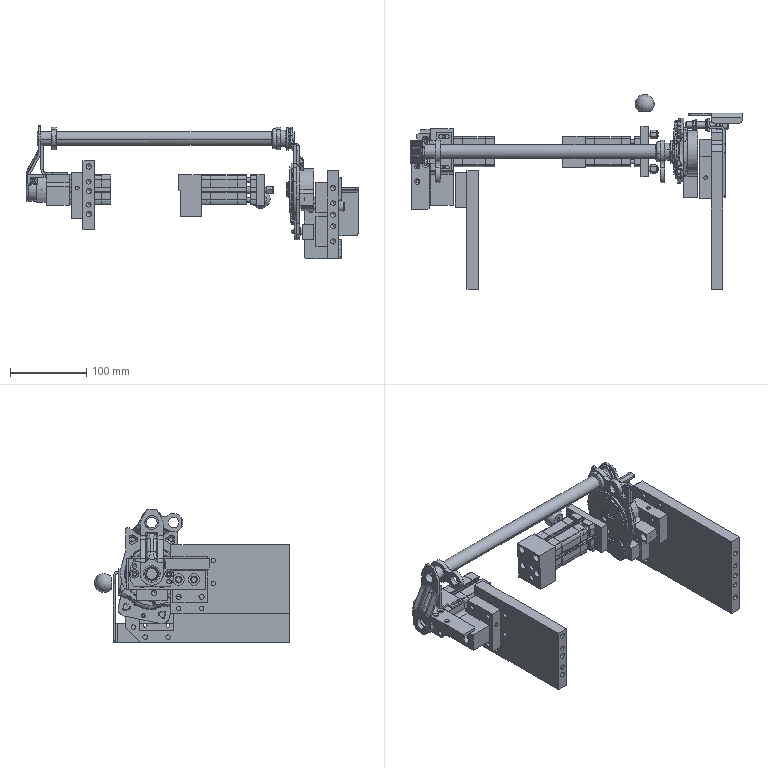Part | NX | features BREP 51 | 56 solids | 3962 faces | volume 1212098 mm3 | plane 1520 | cylinder 1435 | spline 436 | cone 309 | torus 227 | sphere 35 | commonest cylinder face diameters 0.3 x169 0.6 x144 1 x66 0.8 x62 6 x60 1.6 x58